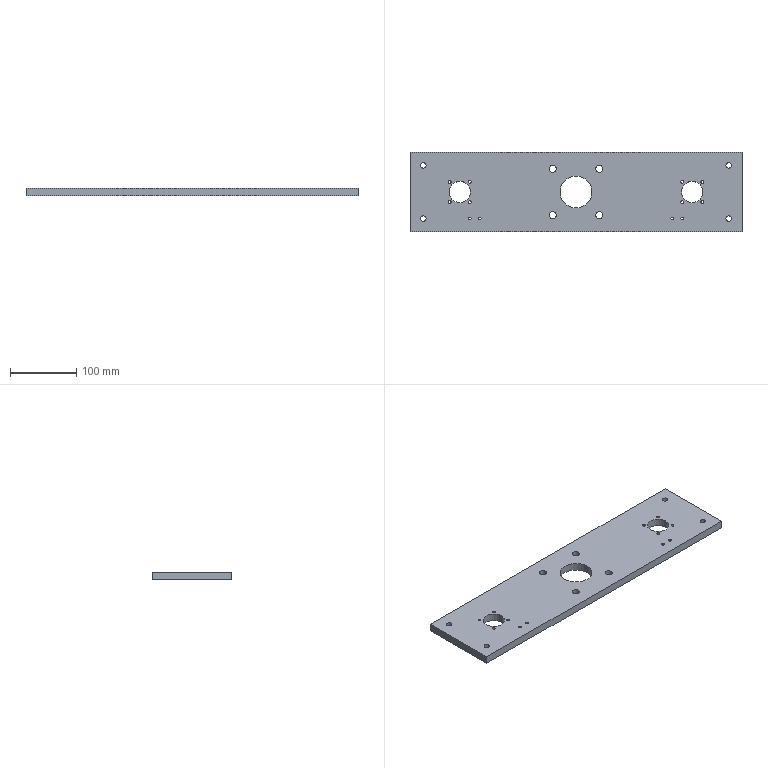Part | STEP file | Hold-down fixture fixing plate | 1 solid | 52 faces | box 500 x 120 x 12 mm | volume 670055 mm3 | cylinder 46 | plane 6 | commonest cylinder face diameters 4.2 x24 8.2 x8 10.5 x8 32.2 x4 48 x2